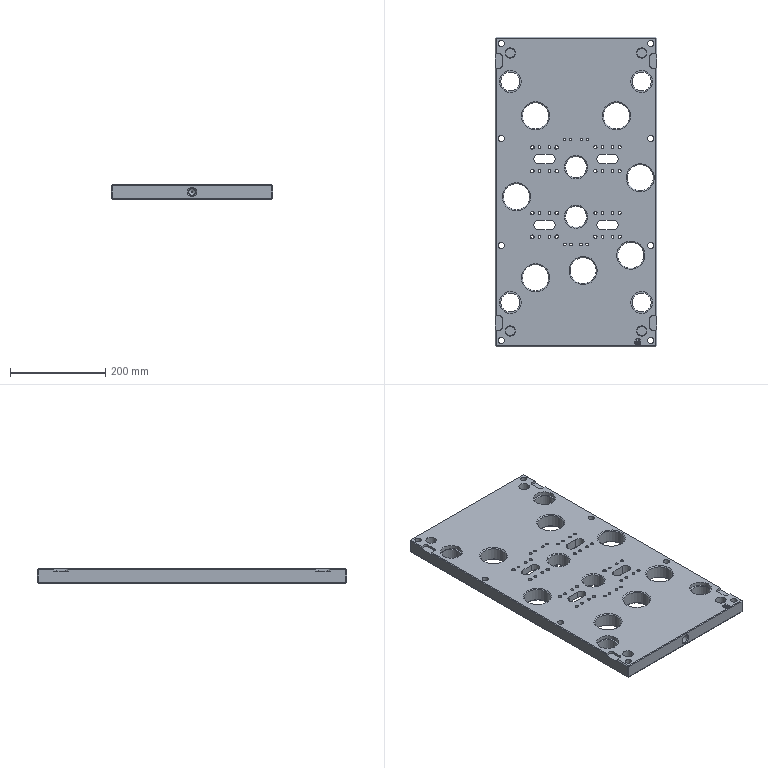Part | STEP file | P011002B003-000 | 1 solid | 608 faces | box 340 x 650 x 30 mm | volume 5385169 mm3 | plane 377 | cylinder 166 | cone 49 | other 16 | commonest cylinder face diameters 10 x24 20 x20 6.8 x19 7.973 x19 8 x19 6 x16